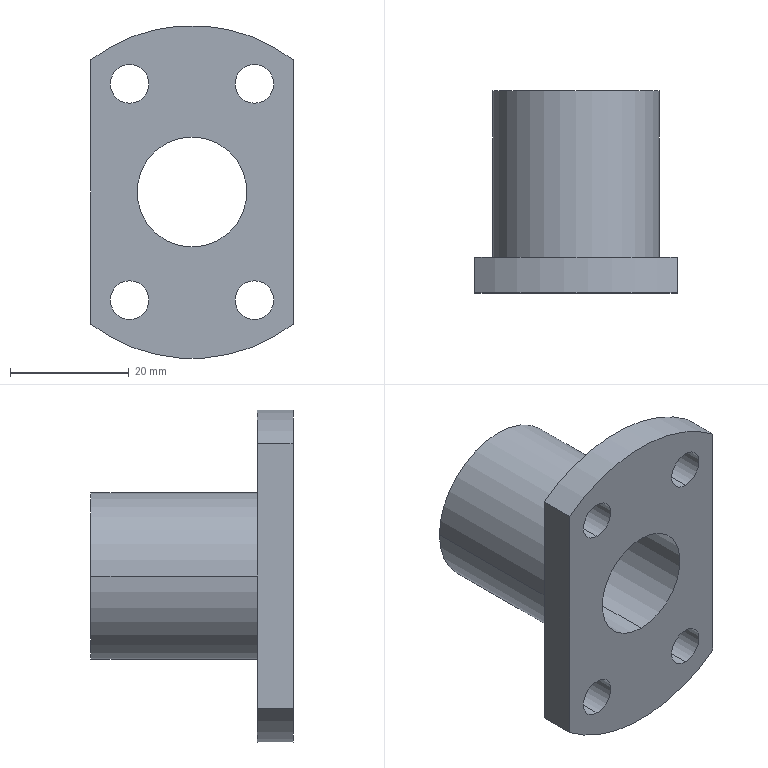Part | SolidWorks | features HoleWzd 2, ICE 1, Revolution 1 | 1 solid | 19 faces | box 34 x 34 x 56 mm | volume 17982 mm3 | cylinder 14 | plane 5 | commonest cylinder face diameters 6.5 x8 18.5 x2 28 x2 56 x2
STEP:
#1=CARTESIAN_POINT('',(0.,34.,9.25));
#2=VERTEX_POINT('',#1);
#3=CARTESIAN_POINT('',(0.,34.,-9.25));
#4=VERTEX_POINT('',#3);
#5=CARTESIAN_POINT('',(0.,34.,0.));
#6=DIRECTION('',(0.,-1.,0.));
#7=DIRECTION('',(1.,0.,0.));
#8=AXIS2_PLACEMENT_3D('',#5,#6,#7);
#9=CIRCLE('',#8,9.25);
#10=EDGE_CURVE('',#2,#4,#9,.T.);
#11=ORIENTED_EDGE('',*,*,#10,.F.);
#12=CARTESIAN_POINT('',(0.,0.,9.25));
#13=VERTEX_POINT('',#12);
#14=CARTESIAN_POINT('',(0.,0.,9.25));
#15=DIRECTION('',(0.,-1.,0.));
#16=VECTOR('',#15,1000.);
#17=LINE('',#14,#16);
#18=EDGE_CURVE('',#2,#13,#17,.T.);
#19=ORIENTED_EDGE('',*,*,#18,.T.);
#20=CARTESIAN_POINT('',(0.,0.,-9.25));
#21=VERTEX_POINT('',#20);
#22=CARTESIAN_POINT('',(0.,0.,0.));
#23=DIRECTION('',(0.,-1.,0.));
#24=DIRECTION('',(0.,0.,-1.));
#25=AXIS2_PLACEMENT_3D('',#22,#23,#24);
#26=CIRCLE('',#25,9.25);
#27=EDGE_CURVE('',#13,#21,#26,.T.);
#28=ORIENTED_EDGE('',*,*,#27,.T.);
#29=CARTESIAN_POINT('',(0.,0.,-9.25));
#30=DIRECTION('',(0.,-1.,0.));
#31=VECTOR('',#30,1000.);
#32=LINE('',#29,#31);
#33=EDGE_CURVE('',#4,#21,#32,.T.);
#34=ORIENTED_EDGE('',*,*,#33,.F.);
#35=EDGE_LOOP('',(#11,#19,#28,#34));
#36=FACE_OUTER_BOUND('',#35,.T.);
#37=CARTESIAN_POINT('',(0.,0.,0.));
#38=DIRECTION('',(0.,-1.,0.));
#39=DIRECTION('',(0.,0.,-1.));
#40=AXIS2_PLACEMENT_3D('',#37,#38,#39);
#41=CYLINDRICAL_SURFACE('',#40,9.25);
#42=ADVANCED_FACE('',(#36),#41,.F.);
#43=CARTESIAN_POINT('',(-10.5,6.,21.437));
#44=VERTEX_POINT('',#43);
#45=CARTESIAN_POINT('',(-10.5,6.,14.937));
#46=VERTEX_POINT('',#45);
#47=CARTESIAN_POINT('',(-10.5,6.,18.187));
#48=DIRECTION('',(0.,-1.,0.));
#49=DIRECTION('',(1.,0.,0.));
#50=AXIS2_PLACEMENT_3D('',#47,#48,#49);
#51=CIRCLE('',#50,3.25);
#52=EDGE_CURVE('',#44,#46,#51,.T.);
#53=ORIENTED_EDGE('',*,*,#52,.F.);
#54=CARTESIAN_POINT('',(-10.5,0.,21.437));
#55=VERTEX_POINT('',#54);
#56=CARTESIAN_POINT('',(-10.5,0.,21.437));
#57=DIRECTION('',(0.,-1.,0.));
#58=VECTOR('',#57,1000.);
#59=LINE('',#56,#58);
#60=EDGE_CURVE('',#44,#55,#59,.T.);
#61=ORIENTED_EDGE('',*,*,#60,.T.);
#62=CARTESIAN_POINT('',(-10.5,0.,14.937));
#63=VERTEX_POINT('',#62);
#64=CARTESIAN_POINT('',(-10.5,0.,18.187));
#65=DIRECTION('',(0.,-1.,0.));
#66=DIRECTION('',(0.,0.,-1.));
#67=AXIS2_PLACEMENT_3D('',#64,#65,#66);
#68=CIRCLE('',#67,3.25);
#69=EDGE_CURVE('',#55,#63,#68,.T.);
#70=ORIENTED_EDGE('',*,*,#69,.T.);
#71=CARTESIAN_POINT('',(-10.5,0.,14.937));
#72=DIRECTION('',(0.,-1.,0.));
#73=VECTOR('',#72,1000.);
#74=LINE('',#71,#73);
#75=EDGE_CURVE('',#46,#63,#74,.T.);
#76=ORIENTED_EDGE('',*,*,#75,.F.);
#77=EDGE_LOOP('',(#53,#61,#70,#76));
#78=FACE_OUTER_BOUND('',#77,.T.);
#79=CARTESIAN_POINT('',(-10.5,0.,18.187));
#80=DIRECTION('',(0.,-1.,0.));
#81=DIRECTION('',(0.,0.,-1.));
#82=AXIS2_PLACEMENT_3D('',#79,#80,#81);
#83=CYLINDRICAL_SURFACE('',#82,3.25);
#84=ADVANCED_FACE('',(#78),#83,.F.);
#85=CARTESIAN_POINT('',(10.5,6.,21.437));
#86=VERTEX_POINT('',#85);
#87=CARTESIAN_POINT('',(10.5,6.,14.937));
#88=VERTEX_POINT('',#87);
#89=CARTESIAN_POINT('',(10.5,6.,18.187));
#90=DIRECTION('',(0.,-1.,0.));
#91=DIRECTION('',(1.,0.,0.));
#92=AXIS2_PLACEMENT_3D('',#89,#90,#91);
#93=CIRCLE('',#92,3.25);
#94=EDGE_CURVE('',#86,#88,#93,.T.);
#95=ORIENTED_EDGE('',*,*,#94,.F.);
#96=CARTESIAN_POINT('',(10.5,0.,21.437));
#97=VERTEX_POINT('',#96);
#98=CARTESIAN_POINT('',(10.5,0.,21.437));
#99=DIRECTION('',(0.,-1.,0.));
#100=VECTOR('',#99,1000.);
#101=LINE('',#98,#100);
#102=EDGE_CURVE('',#86,#97,#101,.T.);
#103=ORIENTED_EDGE('',*,*,#102,.T.);
#104=CARTESIAN_POINT('',(10.5,0.,14.937));
#105=VERTEX_POINT('',#104);
#106=CARTESIAN_POINT('',(10.5,0.,18.187));
#107=DIRECTION('',(0.,-1.,0.));
#108=DIRECTION('',(0.,0.,-1.));
#109=AXIS2_PLACEMENT_3D('',#106,#107,#108);
#110=CIRCLE('',#109,3.25);
#111=EDGE_CURVE('',#97,#105,#110,.T.);
#112=ORIENTED_EDGE('',*,*,#111,.T.);
#113=CARTESIAN_POINT('',(10.5,0.,14.937));
#114=DIRECTION('',(0.,-1.,0.));
#115=VECTOR('',#114,1000.);
#116=LINE('',#113,#115);
#117=EDGE_CURVE('',#88,#105,#116,.T.);
#118=ORIENTED_EDGE('',*,*,#117,.F.);
#119=EDGE_LOOP('',(#95,#103,#112,#118));
#120=FACE_OUTER_BOUND('',#119,.T.);
#121=CARTESIAN_POINT('',(10.5,0.,18.187));
#122=DIRECTION('',(0.,-1.,0.));
#123=DIRECTION('',(0.,0.,-1.));
#124=AXIS2_PLACEMENT_3D('',#121,#122,#123);
#125=CYLINDRICAL_SURFACE('',#124,3.25);
#126=ADVANCED_FACE('',(#120),#125,.F.);
#127=CARTESIAN_POINT('',(-10.5,6.,-14.937));
#128=VERTEX_POINT('',#127);
#129=CARTESIAN_POINT('',(-10.5,6.,-21.437));
#130=VERTEX_POINT('',#129);
#131=CARTESIAN_POINT('',(-10.5,6.,-18.187));
#132=DIRECTION('',(0.,-1.,0.));
#133=DIRECTION('',(1.,0.,0.));
#134=AXIS2_PLACEMENT_3D('',#131,#132,#133);
#135=CIRCLE('',#134,3.25);
#136=EDGE_CURVE('',#128,#130,#135,.T.);
#137=ORIENTED_EDGE('',*,*,#136,.F.);
#138=CARTESIAN_POINT('',(-10.5,0.,-14.937));
#139=VERTEX_POINT('',#138);
#140=CARTESIAN_POINT('',(-10.5,0.,-14.937));
#141=DIRECTION('',(0.,-1.,0.));
#142=VECTOR('',#141,1000.);
#143=LINE('',#140,#142);
#144=EDGE_CURVE('',#128,#139,#143,.T.);
#145=ORIENTED_EDGE('',*,*,#144,.T.);
#146=CARTESIAN_POINT('',(-10.5,0.,-21.437));
#147=VERTEX_POINT('',#146);
#148=CARTESIAN_POINT('',(-10.5,0.,-18.187));
#149=DIRECTION('',(0.,-1.,0.));
#150=DIRECTION('',(0.,0.,-1.));
#151=AXIS2_PLACEMENT_3D('',#148,#149,#150);
#152=CIRCLE('',#151,3.25);
#153=EDGE_CURVE('',#139,#147,#152,.T.);
#154=ORIENTED_EDGE('',*,*,#153,.T.);
#155=CARTESIAN_POINT('',(-10.5,0.,-21.437));
#156=DIRECTION('',(0.,-1.,0.));
#157=VECTOR('',#156,1000.);
#158=LINE('',#155,#157);
#159=EDGE_CURVE('',#130,#147,#158,.T.);
#160=ORIENTED_EDGE('',*,*,#159,.F.);
#161=EDGE_LOOP('',(#137,#145,#154,#160));
#162=FACE_OUTER_BOUND('',#161,.T.);
#163=CARTESIAN_POINT('',(-10.5,0.,-18.187));
#164=DIRECTION('',(0.,-1.,0.));
#165=DIRECTION('',(0.,0.,-1.));
#166=AXIS2_PLACEMENT_3D('',#163,#164,#165);
#167=CYLINDRICAL_SURFACE('',#166,3.25);
#168=ADVANCED_FACE('',(#162),#167,.F.);
#169=CARTESIAN_POINT('',(10.5,6.,-14.937));
#170=VERTEX_POINT('',#169);
#171=CARTESIAN_POINT('',(10.5,6.,-21.437));
#172=VERTEX_POINT('',#171);
#173=CARTESIAN_POINT('',(10.5,6.,-18.187));
#174=DIRECTION('',(0.,-1.,0.));
#175=DIRECTION('',(1.,0.,0.));
#176=AXIS2_PLACEMENT_3D('',#173,#174,#175);
#177=CIRCLE('',#176,3.25);
#178=EDGE_CURVE('',#170,#172,#177,.T.);
#179=ORIENTED_EDGE('',*,*,#178,.F.);
#180=CARTESIAN_POINT('',(10.5,0.,-14.937));
#181=VERTEX_POINT('',#180);
#182=CARTESIAN_POINT('',(10.5,0.,-14.937));
#183=DIRECTION('',(0.,-1.,0.));
#184=VECTOR('',#183,1000.);
#185=LINE('',#182,#184);
#186=EDGE_CURVE('',#170,#181,#185,.T.);
#187=ORIENTED_EDGE('',*,*,#186,.T.);
#188=CARTESIAN_POINT('',(10.5,0.,-21.437));
#189=VERTEX_POINT('',#188);
#190=CARTESIAN_POINT('',(10.5,0.,-18.187));
#191=DIRECTION('',(0.,-1.,0.));
#192=DIRECTION('',(0.,0.,-1.));
#193=AXIS2_PLACEMENT_3D('',#190,#191,#192);
#194=CIRCLE('',#193,3.25);
#195=EDGE_CURVE('',#181,#189,#194,.T.);
#196=ORIENTED_EDGE('',*,*,#195,.T.);
#197=CARTESIAN_POINT('',(10.5,0.,-21.437));
#198=DIRECTION('',(0.,-1.,0.));
#199=VECTOR('',#198,1000.);
#200=LINE('',#197,#199);
#201=EDGE_CURVE('',#172,#189,#200,.T.);
#202=ORIENTED_EDGE('',*,*,#201,.F.);
#203=EDGE_LOOP('',(#179,#187,#196,#202));
#204=FACE_OUTER_BOUND('',#203,.T.);
#205=CARTESIAN_POINT('',(10.5,0.,-18.187));
#206=DIRECTION('',(0.,-1.,0.));
#207=DIRECTION('',(0.,0.,-1.));
#208=AXIS2_PLACEMENT_3D('',#205,#206,#207);
#209=CYLINDRICAL_SURFACE('',#208,3.25);
#210=ADVANCED_FACE('',(#204),#209,.F.);
#211=CARTESIAN_POINT('',(-14.,6.,0.));
#212=VERTEX_POINT('',#211);
#213=CARTESIAN_POINT('',(14.,6.,0.));
#214=VERTEX_POINT('',#213);
#215=CARTESIAN_POINT('',(0.,6.,0.));
#216=DIRECTION('',(0.,1.,0.));
#217=DIRECTION('',(-1.,0.,0.));
#218=AXIS2_PLACEMENT_3D('',#215,#216,#217);
#219=CIRCLE('',#218,14.);
#220=EDGE_CURVE('',#212,#214,#219,.T.);
#221=ORIENTED_EDGE('',*,*,#220,.T.);
#222=CARTESIAN_POINT('',(14.,34.,0.));
#223=VERTEX_POINT('',#222);
#224=CARTESIAN_POINT('',(14.,34.,0.));
#225=DIRECTION('',(0.,1.,0.));
#226=VECTOR('',#225,1000.);
#227=LINE('',#224,#226);
#228=EDGE_CURVE('',#214,#223,#227,.T.);
#229=ORIENTED_EDGE('',*,*,#228,.T.);
#230=CARTESIAN_POINT('',(-14.,34.,0.));
#231=VERTEX_POINT('',#230);
#232=CARTESIAN_POINT('',(0.,34.,0.));
#233=DIRECTION('',(0.,1.,0.));
#234=DIRECTION('',(-1.,0.,0.));
#235=AXIS2_PLACEMENT_3D('',#232,#233,#234);
#236=CIRCLE('',#235,14.);
#237=EDGE_CURVE('',#231,#223,#236,.T.);
#238=ORIENTED_EDGE('',*,*,#237,.F.);
#239=CARTESIAN_POINT('',(-14.,34.,0.));
#240=DIRECTION('',(0.,1.,0.));
#241=VECTOR('',#240,1000.);
#242=LINE('',#239,#241);
#243=EDGE_CURVE('',#212,#231,#242,.T.);
#244=ORIENTED_EDGE('',*,*,#243,.F.);
#245=EDGE_LOOP('',(#221,#229,#238,#244));
#246=FACE_OUTER_BOUND('',#245,.T.);
#247=CARTESIAN_POINT('',(0.,34.,0.));
#248=DIRECTION('',(0.,1.,0.));
#249=DIRECTION('',(-1.,0.,0.));
#250=AXIS2_PLACEMENT_3D('',#247,#248,#249);
#251=CYLINDRICAL_SURFACE('',#250,14.);
#252=ADVANCED_FACE('',(#246),#251,.T.);
#253=CARTESIAN_POINT('',(0.,0.,0.));
#254=DIRECTION('',(0.,-1.,0.));
#255=DIRECTION('',(0.,0.,-1.));
#256=AXIS2_PLACEMENT_3D('',#253,#254,#255);
#257=CIRCLE('',#256,9.25);
#258=EDGE_CURVE('',#21,#13,#257,.T.);
#259=ORIENTED_EDGE('',*,*,#258,.F.);
#260=ORIENTED_EDGE('',*,*,#27,.F.);
#261=EDGE_LOOP('',(#259,#260));
#262=FACE_BOUND('',#261,.T.);
#263=CARTESIAN_POINT('',(-10.5,0.,18.187));
#264=DIRECTION('',(0.,-1.,0.));
#265=DIRECTION('',(0.,0.,-1.));
#266=AXIS2_PLACEMENT_3D('',#263,#264,#265);
#267=CIRCLE('',#266,3.25);
#268=EDGE_CURVE('',#63,#55,#267,.T.);
#269=ORIENTED_EDGE('',*,*,#268,.F.);
#270=ORIENTED_EDGE('',*,*,#69,.F.);
#271=EDGE_LOOP('',(#269,#270));
#272=FACE_BOUND('',#271,.T.);
#273=CARTESIAN_POINT('',(10.5,0.,18.187));
#274=DIRECTION('',(0.,-1.,0.));
#275=DIRECTION('',(0.,0.,-1.));
#276=AXIS2_PLACEMENT_3D('',#273,#274,#275);
#277=CIRCLE('',#276,3.25);
#278=EDGE_CURVE('',#105,#97,#277,.T.);
#279=ORIENTED_EDGE('',*,*,#278,.F.);
#280=ORIENTED_EDGE('',*,*,#111,.F.);
#281=EDGE_LOOP('',(#279,#280));
#282=FACE_BOUND('',#281,.T.);
#283=CARTESIAN_POINT('',(-10.5,0.,-18.187));
#284=DIRECTION('',(0.,-1.,0.));
#285=DIRECTION('',(0.,0.,-1.));
#286=AXIS2_PLACEMENT_3D('',#283,#284,#285);
#287=CIRCLE('',#286,3.25);
#288=EDGE_CURVE('',#147,#139,#287,.T.);
#289=ORIENTED_EDGE('',*,*,#288,.F.);
#290=ORIENTED_EDGE('',*,*,#153,.F.);
#291=EDGE_LOOP('',(#289,#290));
#292=FACE_BOUND('',#291,.T.);
#293=CARTESIAN_POINT('',(10.5,0.,-18.187));
#294=DIRECTION('',(0.,-1.,0.));
#295=DIRECTION('',(0.,0.,-1.));
#296=AXIS2_PLACEMENT_3D('',#293,#294,#295);
#297=CIRCLE('',#296,3.25);
#298=EDGE_CURVE('',#189,#181,#297,.T.);
#299=ORIENTED_EDGE('',*,*,#298,.F.);
#300=ORIENTED_EDGE('',*,*,#195,.F.);
#301=EDGE_LOOP('',(#299,#300));
#302=FACE_BOUND('',#301,.T.);
#303=CARTESIAN_POINT('',(-17.,0.,22.249));
#304=VERTEX_POINT('',#303);
#305=CARTESIAN_POINT('',(-17.,0.,-22.249));
#306=VERTEX_POINT('',#305);
#307=CARTESIAN_POINT('',(-17.,0.,30.));
#308=DIRECTION('',(0.,0.,-1.));
#309=VECTOR('',#308,1000.);
#310=LINE('',#307,#309);
#311=EDGE_CURVE('',#304,#306,#310,.T.);
#312=ORIENTED_EDGE('',*,*,#311,.T.);
#313=CARTESIAN_POINT('',(17.,0.,-22.249));
#314=VERTEX_POINT('',#313);
#315=CARTESIAN_POINT('',(0.,0.,0.));
#316=DIRECTION('',(0.,1.,0.));
#317=DIRECTION('',(-1.,0.,0.));
#318=AXIS2_PLACEMENT_3D('',#315,#316,#317);
#319=CIRCLE('',#318,28.);
#320=EDGE_CURVE('',#314,#306,#319,.T.);
#321=ORIENTED_EDGE('',*,*,#320,.F.);
#322=CARTESIAN_POINT('',(17.,0.,22.249));
#323=VERTEX_POINT('',#322);
#324=CARTESIAN_POINT('',(17.,0.,30.));
#325=DIRECTION('',(0.,0.,1.));
#326=VECTOR('',#325,1000.);
#327=LINE('',#324,#326);
#328=EDGE_CURVE('',#314,#323,#327,.T.);
#329=ORIENTED_EDGE('',*,*,#328,.T.);
#330=CARTESIAN_POINT('',(0.,0.,0.));
#331=DIRECTION('',(0.,1.,0.));
#332=DIRECTION('',(-1.,0.,0.));
#333=AXIS2_PLACEMENT_3D('',#330,#331,#332);
#334=CIRCLE('',#333,28.);
#335=EDGE_CURVE('',#304,#323,#334,.T.);
#336=ORIENTED_EDGE('',*,*,#335,.F.);
#337=EDGE_LOOP('',(#312,#321,#329,#336));
#338=FACE_OUTER_BOUND('',#337,.T.);
#339=CARTESIAN_POINT('',(0.,0.,0.));
#340=DIRECTION('',(0.,1.,0.));
#341=DIRECTION('',(-1.,0.,0.));
#342=AXIS2_PLACEMENT_3D('',#339,#340,#341);
#343=PLANE('',#342);
#344=ADVANCED_FACE('',(#262,#272,#282,#292,#302,#338),#343,.F.);
#345=CARTESIAN_POINT('',(-17.,6.,22.249));
#346=VERTEX_POINT('',#345);
#347=CARTESIAN_POINT('',(-17.,34.,22.249));
#348=DIRECTION('',(0.,1.,0.));
#349=VECTOR('',#348,1000.);
#350=LINE('',#347,#349);
#351=EDGE_CURVE('',#304,#346,#350,.T.);
#352=ORIENTED_EDGE('',*,*,#351,.F.);
#353=ORIENTED_EDGE('',*,*,#335,.T.);
#354=CARTESIAN_POINT('',(17.,6.,22.249));
#355=VERTEX_POINT('',#354);
#356=CARTESIAN_POINT('',(17.,34.,22.249));
#357=DIRECTION('',(0.,-1.,0.));
#358=VECTOR('',#357,1000.);
#359=LINE('',#356,#358);
#360=EDGE_CURVE('',#355,#323,#359,.T.);
#361=ORIENTED_EDGE('',*,*,#360,.F.);
#362=CARTESIAN_POINT('',(0.,6.,0.));
#363=DIRECTION('',(0.,1.,0.));
#364=DIRECTION('',(-1.,0.,0.));
#365=AXIS2_PLACEMENT_3D('',#362,#363,#364);
#366=CIRCLE('',#365,28.);
#367=EDGE_CURVE('',#346,#355,#366,.T.);
#368=ORIENTED_EDGE('',*,*,#367,.F.);
#369=EDGE_LOOP('',(#352,#353,#361,#368));
#370=FACE_OUTER_BOUND('',#369,.T.);
#371=CARTESIAN_POINT('',(0.,34.,0.));
#372=DIRECTION('',(0.,1.,0.));
#373=DIRECTION('',(-1.,0.,0.));
#374=AXIS2_PLACEMENT_3D('',#371,#372,#373);
#375=CYLINDRICAL_SURFACE('',#374,28.);
#376=ADVANCED_FACE('',(#370),#375,.T.);
#377=CARTESIAN_POINT('',(-17.,6.,-22.249));
#378=VERTEX_POINT('',#377);
#379=CARTESIAN_POINT('',(-17.,34.,-22.249));
#380=DIRECTION('',(0.,-1.,0.));
#381=VECTOR('',#380,1000.);
#382=LINE('',#379,#381);
#383=EDGE_CURVE('',#378,#306,#382,.T.);
#384=ORIENTED_EDGE('',*,*,#383,.F.);
#385=CARTESIAN_POINT('',(17.,6.,-22.249));
#386=VERTEX_POINT('',#385);
#387=CARTESIAN_POINT('',(0.,6.,0.));
#388=DIRECTION('',(0.,1.,0.));
#389=DIRECTION('',(-1.,0.,0.));
#390=AXIS2_PLACEMENT_3D('',#387,#388,#389);
#391=CIRCLE('',#390,28.);
#392=EDGE_CURVE('',#386,#378,#391,.T.);
#393=ORIENTED_EDGE('',*,*,#392,.F.);
#394=CARTESIAN_POINT('',(17.,34.,-22.249));
#395=DIRECTION('',(0.,1.,0.));
#396=VECTOR('',#395,1000.);
#397=LINE('',#394,#396);
#398=EDGE_CURVE('',#314,#386,#397,.T.);
#399=ORIENTED_EDGE('',*,*,#398,.F.);
#400=ORIENTED_EDGE('',*,*,#320,.T.);
#401=EDGE_LOOP('',(#384,#393,#399,#400));
#402=FACE_OUTER_BOUND('',#401,.T.);
#403=CARTESIAN_POINT('',(0.,34.,0.));
#404=DIRECTION('',(0.,1.,0.));
#405=DIRECTION('',(-1.,0.,0.));
#406=AXIS2_PLACEMENT_3D('',#403,#404,#405);
#407=CYLINDRICAL_SURFACE('',#406,28.);
#408=ADVANCED_FACE('',(#402),#407,.T.);
#409=CARTESIAN_POINT('',(-10.5,6.,18.187));
#410=DIRECTION('',(0.,-1.,0.));
#411=DIRECTION('',(1.,0.,0.));
#412=AXIS2_PLACEMENT_3D('',#409,#410,#411);
#413=CIRCLE('',#412,3.25);
#414=EDGE_CURVE('',#46,#44,#413,.T.);
#415=ORIENTED_EDGE('',*,*,#414,.T.);
#416=ORIENTED_EDGE('',*,*,#52,.T.);
#417=EDGE_LOOP('',(#415,#416));
#418=FACE_BOUND('',#417,.T.);
#419=CARTESIAN_POINT('',(10.5,6.,18.187));
#420=DIRECTION('',(0.,-1.,0.));
#421=DIRECTION('',(1.,0.,0.));
#422=AXIS2_PLACEMENT_3D('',#419,#420,#421);
#423=CIRCLE('',#422,3.25);
#424=EDGE_CURVE('',#88,#86,#423,.T.);
#425=ORIENTED_EDGE('',*,*,#424,.T.);
#426=ORIENTED_EDGE('',*,*,#94,.T.);
#427=EDGE_LOOP('',(#425,#426));
#428=FACE_BOUND('',#427,.T.);
#429=CARTESIAN_POINT('',(-10.5,6.,-18.187));
#430=DIRECTION('',(0.,-1.,0.));
#431=DIRECTION('',(1.,0.,0.));
#432=AXIS2_PLACEMENT_3D('',#429,#430,#431);
#433=CIRCLE('',#432,3.25);
#434=EDGE_CURVE('',#130,#128,#433,.T.);
#435=ORIENTED_EDGE('',*,*,#434,.T.);
#436=ORIENTED_EDGE('',*,*,#136,.T.);
#437=EDGE_LOOP('',(#435,#436));
#438=FACE_BOUND('',#437,.T.);
#439=CARTESIAN_POINT('',(10.5,6.,-18.187));
#440=DIRECTION('',(0.,-1.,0.));
#441=DIRECTION('',(1.,0.,0.));
#442=AXIS2_PLACEMENT_3D('',#439,#440,#441);
#443=CIRCLE('',#442,3.25);
#444=EDGE_CURVE('',#172,#170,#443,.T.);
#445=ORIENTED_EDGE('',*,*,#444,.T.);
#446=ORIENTED_EDGE('',*,*,#178,.T.);
#447=EDGE_LOOP('',(#445,#446));
#448=FACE_BOUND('',#447,.T.);
#449=ORIENTED_EDGE('',*,*,#220,.F.);
#450=CARTESIAN_POINT('',(0.,6.,0.));
#451=DIRECTION('',(0.,1.,0.));
#452=DIRECTION('',(-1.,0.,0.));
#453=AXIS2_PLACEMENT_3D('',#450,#451,#452);
#454=CIRCLE('',#453,14.);
#455=EDGE_CURVE('',#214,#212,#454,.T.);
#456=ORIENTED_EDGE('',*,*,#455,.F.);
#457=EDGE_LOOP('',(#449,#456));
#458=FACE_BOUND('',#457,.T.);
#459=CARTESIAN_POINT('',(-17.,6.,0.));
#460=DIRECTION('',(0.,0.,-1.));
#461=VECTOR('',#460,1000.);
#462=LINE('',#459,#461);
#463=EDGE_CURVE('',#346,#378,#462,.T.);
#464=ORIENTED_EDGE('',*,*,#463,.F.);
#465=ORIENTED_EDGE('',*,*,#367,.T.);
#466=CARTESIAN_POINT('',(17.,6.,0.));
#467=DIRECTION('',(0.,0.,1.));
#468=VECTOR('',#467,1000.);
#469=LINE('',#466,#468);
#470=EDGE_CURVE('',#386,#355,#469,.T.);
#471=ORIENTED_EDGE('',*,*,#470,.F.);
#472=ORIENTED_EDGE('',*,*,#392,.T.);
#473=EDGE_LOOP('',(#464,#465,#471,#472));
#474=FACE_OUTER_BOUND('',#473,.T.);
#475=CARTESIAN_POINT('',(28.,6.,0.));
#476=DIRECTION('',(0.,-1.,0.));
#477=DIRECTION('',(1.,0.,0.));
#478=AXIS2_PLACEMENT_3D('',#475,#476,#477);
#479=PLANE('',#478);
#480=ADVANCED_FACE('',(#418,#428,#438,#448,#458,#474),#479,.F.);
#481=ORIENTED_EDGE('',*,*,#228,.F.);
#482=ORIENTED_EDGE('',*,*,#455,.T.);
#483=ORIENTED_EDGE('',*,*,#243,.T.);
#484=CARTESIAN_POINT('',(0.,34.,0.));
#485=DIRECTION('',(0.,1.,0.));
#486=DIRECTION('',(-1.,0.,0.));
#487=AXIS2_PLACEMENT_3D('',#484,#485,#486);
#488=CIRCLE('',#487,14.);
#489=EDGE_CURVE('',#223,#231,#488,.T.);
#490=ORIENTED_EDGE('',*,*,#489,.F.);
#491=EDGE_LOOP('',(#481,#482,#483,#490));
#492=FACE_OUTER_BOUND('',#491,.T.);
#493=CARTESIAN_POINT('',(0.,34.,0.));
#494=DIRECTION('',(0.,1.,0.));
#495=DIRECTION('',(-1.,0.,0.));
#496=AXIS2_PLACEMENT_3D('',#493,#494,#495);
#497=CYLINDRICAL_SURFACE('',#496,14.);
#498=ADVANCED_FACE('',(#492),#497,.T.);
#499=CARTESIAN_POINT('',(0.,34.,0.));
#500=DIRECTION('',(0.,-1.,0.));
#501=DIRECTION('',(1.,0.,0.));
#502=AXIS2_PLACEMENT_3D('',#499,#500,#501);
#503=CIRCLE('',#502,9.25);
#504=EDGE_CURVE('',#4,#2,#503,.T.);
#505=ORIENTED_EDGE('',*,*,#504,.T.);
#506=ORIENTED_EDGE('',*,*,#10,.T.);
#507=EDGE_LOOP('',(#505,#506));
#508=FACE_BOUND('',#507,.T.);
#509=ORIENTED_EDGE('',*,*,#237,.T.);
#510=ORIENTED_EDGE('',*,*,#489,.T.);
#511=EDGE_LOOP('',(#509,#510));
#512=FACE_OUTER_BOUND('',#511,.T.);
#513=CARTESIAN_POINT('',(14.,34.,0.));
#514=DIRECTION('',(0.,-1.,0.));
#515=DIRECTION('',(1.,0.,0.));
#516=AXIS2_PLACEMENT_3D('',#513,#514,#515);
#517=PLANE('',#516);
#518=ADVANCED_FACE('',(#508,#512),#517,.F.);
#519=ORIENTED_EDGE('',*,*,#398,.T.);
#520=ORIENTED_EDGE('',*,*,#470,.T.);
#521=ORIENTED_EDGE('',*,*,#360,.T.);
#522=ORIENTED_EDGE('',*,*,#328,.F.);
#523=EDGE_LOOP('',(#519,#520,#521,#522));
#524=FACE_OUTER_BOUND('',#523,.T.);
#525=CARTESIAN_POINT('',(17.,10.,30.));
#526=DIRECTION('',(1.,0.,0.));
#527=DIRECTION('',(0.,0.,-1.));
#528=AXIS2_PLACEMENT_3D('',#525,#526,#527);
#529=PLANE('',#528);
#530=ADVANCED_FACE('',(#524),#529,.T.);
#531=ORIENTED_EDGE('',*,*,#351,.T.);
#532=ORIENTED_EDGE('',*,*,#463,.T.);
#533=ORIENTED_EDGE('',*,*,#383,.T.);
#534=ORIENTED_EDGE('',*,*,#311,.F.);
#535=EDGE_LOOP('',(#531,#532,#533,#534));
#536=FACE_OUTER_BOUND('',#535,.T.);
#537=CARTESIAN_POINT('',(-17.,10.,30.));
#538=DIRECTION('',(-1.,0.,0.));
#539=DIRECTION('',(0.,0.,1.));
#540=AXIS2_PLACEMENT_3D('',#537,#538,#539);
#541=PLANE('',#540);
#542=ADVANCED_FACE('',(#536),#541,.T.);
#543=ORIENTED_EDGE('',*,*,#186,.F.);
#544=ORIENTED_EDGE('',*,*,#444,.F.);
#545=ORIENTED_EDGE('',*,*,#201,.T.);
#546=ORIENTED_EDGE('',*,*,#298,.T.);
#547=EDGE_LOOP('',(#543,#544,#545,#546));
#548=FACE_OUTER_BOUND('',#547,.T.);
#549=CARTESIAN_POINT('',(10.5,0.,-18.187));
#550=DIRECTION('',(0.,-1.,0.));
#551=DIRECTION('',(0.,0.,-1.));
#552=AXIS2_PLACEMENT_3D('',#549,#550,#551);
#553=CYLINDRICAL_SURFACE('',#552,3.25);
#554=ADVANCED_FACE('',(#548),#553,.F.);
#555=ORIENTED_EDGE('',*,*,#144,.F.);
#556=ORIENTED_EDGE('',*,*,#434,.F.);
#557=ORIENTED_EDGE('',*,*,#159,.T.);
#558=ORIENTED_EDGE('',*,*,#288,.T.);
#559=EDGE_LOOP('',(#555,#556,#557,#558));
#560=FACE_OUTER_BOUND('',#559,.T.);
#561=CARTESIAN_POINT('',(-10.5,0.,-18.187));
#562=DIRECTION('',(0.,-1.,0.));
#563=DIRECTION('',(0.,0.,-1.));
#564=AXIS2_PLACEMENT_3D('',#561,#562,#563);
#565=CYLINDRICAL_SURFACE('',#564,3.25);
#566=ADVANCED_FACE('',(#560),#565,.F.);
#567=ORIENTED_EDGE('',*,*,#102,.F.);
#568=ORIENTED_EDGE('',*,*,#424,.F.);
#569=ORIENTED_EDGE('',*,*,#117,.T.);
#570=ORIENTED_EDGE('',*,*,#278,.T.);
#571=EDGE_LOOP('',(#567,#568,#569,#570));
#572=FACE_OUTER_BOUND('',#571,.T.);
#573=CARTESIAN_POINT('',(10.5,0.,18.187));
#574=DIRECTION('',(0.,-1.,0.));
#575=DIRECTION('',(0.,0.,-1.));
#576=AXIS2_PLACEMENT_3D('',#573,#574,#575);
#577=CYLINDRICAL_SURFACE('',#576,3.25);
#578=ADVANCED_FACE('',(#572),#577,.F.);
#579=ORIENTED_EDGE('',*,*,#60,.F.);
#580=ORIENTED_EDGE('',*,*,#414,.F.);
#581=ORIENTED_EDGE('',*,*,#75,.T.);
#582=ORIENTED_EDGE('',*,*,#268,.T.);
#583=EDGE_LOOP('',(#579,#580,#581,#582));
#584=FACE_OUTER_BOUND('',#583,.T.);
#585=CARTESIAN_POINT('',(-10.5,0.,18.187));
#586=DIRECTION('',(0.,-1.,0.));
#587=DIRECTION('',(0.,0.,-1.));
#588=AXIS2_PLACEMENT_3D('',#585,#586,#587);
#589=CYLINDRICAL_SURFACE('',#588,3.25);
#590=ADVANCED_FACE('',(#584),#589,.F.);
#591=ORIENTED_EDGE('',*,*,#18,.F.);
#592=ORIENTED_EDGE('',*,*,#504,.F.);
#593=ORIENTED_EDGE('',*,*,#33,.T.);
#594=ORIENTED_EDGE('',*,*,#258,.T.);
#595=EDGE_LOOP('',(#591,#592,#593,#594));
#596=FACE_OUTER_BOUND('',#595,.T.);
#597=CARTESIAN_POINT('',(0.,0.,0.));
#598=DIRECTION('',(0.,-1.,0.));
#599=DIRECTION('',(0.,0.,-1.));
#600=AXIS2_PLACEMENT_3D('',#597,#598,#599);
#601=CYLINDRICAL_SURFACE('',#600,9.25);
#602=ADVANCED_FACE('',(#596),#601,.F.);
#603=CLOSED_SHELL('',(#42,#84,#126,#168,#210,#252,#344,#376,#408,#480,#498,#518,#530,#542,#554,#566,#578,#590,#602));
#604=MANIFOLD_SOLID_BREP('',#603);
#605=CARTESIAN_POINT('',(0.,0.,0.));
#606=DIRECTION('',(0.,0.,1.));
#607=DIRECTION('',(1.,0.,0.));
#608=AXIS2_PLACEMENT_3D('',#605,#606,#607);
#609=(LENGTH_UNIT()NAMED_UNIT(*)SI_UNIT(.MILLI.,.METRE.));
#610=UNCERTAINTY_MEASURE_WITH_UNIT(LENGTH_MEASURE(0.00001),#609,'','');
#611=(NAMED_UNIT(*)PLANE_ANGLE_UNIT()SI_UNIT($,.RADIAN.));
#612=(NAMED_UNIT(*)SI_UNIT($,.STERADIAN.)SOLID_ANGLE_UNIT());
#613=(GEOMETRIC_REPRESENTATION_CONTEXT(3)GLOBAL_UNCERTAINTY_ASSIGNED_CONTEXT((#610))GLOBAL_UNIT_ASSIGNED_CONTEXT((#609,#611,#612))REPRESENTATION_CONTEXT('',''));
#614=ADVANCED_BREP_SHAPE_REPRESENTATION('',(#604,#608),#613);